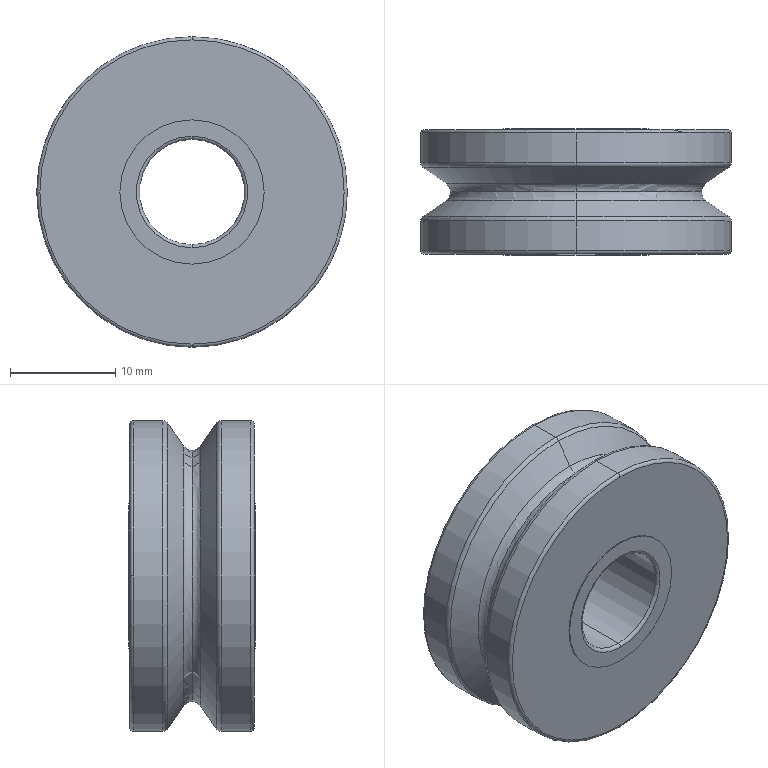Part | SolidWorks | features BaseBody 1 | 1 solid | 34 faces | box 29.5 x 12 x 29.5 mm | volume 6423 mm3 | torus 16 | cylinder 10 | cone 4 | plane 4 | commonest cylinder face diameters 13.7 x4 29.5 x4 10 x2
STEP:
#1=CARTESIAN_POINT('',(0.,-0.8192,-12.35));
#2=VERTEX_POINT('',#1);
#3=CARTESIAN_POINT('',(0.,0.,-11.923));
#4=VERTEX_POINT('',#3);
#5=CARTESIAN_POINT('',(0.,0.,-12.923));
#6=DIRECTION('',(-1.,0.,0.));
#7=DIRECTION('',(0.,0.,1.));
#8=AXIS2_PLACEMENT_3D('',#5,#6,#7);
#9=CIRCLE('',#8,1.);
#10=EDGE_CURVE('',#2,#4,#9,.T.);
#11=ORIENTED_EDGE('',*,*,#10,.T.);
#12=CARTESIAN_POINT('',(0.,0.,11.923));
#13=VERTEX_POINT('',#12);
#14=CARTESIAN_POINT('',(0.,0.,0.));
#15=DIRECTION('',(0.,-1.,0.));
#16=DIRECTION('',(0.,0.,-1.));
#17=AXIS2_PLACEMENT_3D('',#14,#15,#16);
#18=CIRCLE('',#17,11.923);
#19=EDGE_CURVE('',#4,#13,#18,.T.);
#20=ORIENTED_EDGE('',*,*,#19,.T.);
#21=CARTESIAN_POINT('',(0.,-0.8192,12.35));
#22=VERTEX_POINT('',#21);
#23=CARTESIAN_POINT('',(0.,0.,12.923));
#24=DIRECTION('',(1.,0.,0.));
#25=DIRECTION('',(0.,0.,-1.));
#26=AXIS2_PLACEMENT_3D('',#23,#24,#25);
#27=CIRCLE('',#26,1.);
#28=EDGE_CURVE('',#22,#13,#27,.T.);
#29=ORIENTED_EDGE('',*,*,#28,.F.);
#30=CARTESIAN_POINT('',(0.,-0.8192,0.));
#31=DIRECTION('',(0.,-1.,0.));
#32=DIRECTION('',(0.,0.,-1.));
#33=AXIS2_PLACEMENT_3D('',#30,#31,#32);
#34=CIRCLE('',#33,12.35);
#35=EDGE_CURVE('',#2,#22,#34,.T.);
#36=ORIENTED_EDGE('',*,*,#35,.F.);
#37=EDGE_LOOP('',(#11,#20,#29,#36));
#38=FACE_OUTER_BOUND('',#37,.T.);
#39=CARTESIAN_POINT('',(0.,0.,0.));
#40=DIRECTION('',(0.,-1.,0.));
#41=DIRECTION('',(0.,0.,-1.));
#42=AXIS2_PLACEMENT_3D('',#39,#40,#41);
#43=TOROIDAL_SURFACE('',#42,12.923,1.);
#44=ADVANCED_FACE('',(#38),#43,.F.);
#45=ORIENTED_EDGE('',*,*,#28,.T.);
#46=CARTESIAN_POINT('',(0.,0.,0.));
#47=DIRECTION('',(0.,-1.,0.));
#48=DIRECTION('',(0.,0.,-1.));
#49=AXIS2_PLACEMENT_3D('',#46,#47,#48);
#50=CIRCLE('',#49,11.923);
#51=EDGE_CURVE('',#13,#4,#50,.T.);
#52=ORIENTED_EDGE('',*,*,#51,.T.);
#53=ORIENTED_EDGE('',*,*,#10,.F.);
#54=CARTESIAN_POINT('',(0.,-0.8192,0.));
#55=DIRECTION('',(0.,-1.,0.));
#56=DIRECTION('',(0.,0.,-1.));
#57=AXIS2_PLACEMENT_3D('',#54,#55,#56);
#58=CIRCLE('',#57,12.35);
#59=EDGE_CURVE('',#22,#2,#58,.T.);
#60=ORIENTED_EDGE('',*,*,#59,.F.);
#61=EDGE_LOOP('',(#45,#52,#53,#60));
#62=FACE_OUTER_BOUND('',#61,.T.);
#63=CARTESIAN_POINT('',(0.,0.,0.));
#64=DIRECTION('',(0.,-1.,0.));
#65=DIRECTION('',(0.,0.,-1.));
#66=AXIS2_PLACEMENT_3D('',#63,#64,#65);
#67=TOROIDAL_SURFACE('',#66,12.923,1.);
#68=ADVANCED_FACE('',(#62),#67,.F.);
#69=CARTESIAN_POINT('',(0.,5.9,14.45));
#70=VERTEX_POINT('',#69);
#71=CARTESIAN_POINT('',(-14.45,5.9,0.));
#72=VERTEX_POINT('',#71);
#73=CARTESIAN_POINT('',(0.,5.9,0.));
#74=DIRECTION('',(0.,-1.,0.));
#75=DIRECTION('',(1.,0.,0.));
#76=AXIS2_PLACEMENT_3D('',#73,#74,#75);
#77=CIRCLE('',#76,14.45);
#78=EDGE_CURVE('',#70,#72,#77,.T.);
#79=ORIENTED_EDGE('',*,*,#78,.T.);
#80=CARTESIAN_POINT('',(-14.75,5.6,0.));
#81=VERTEX_POINT('',#80);
#82=CARTESIAN_POINT('',(-14.45,5.6,0.));
#83=DIRECTION('',(0.,0.,1.));
#84=DIRECTION('',(1.,0.,0.));
#85=AXIS2_PLACEMENT_3D('',#82,#83,#84);
#86=CIRCLE('',#85,0.3);
#87=EDGE_CURVE('',#72,#81,#86,.T.);
#88=ORIENTED_EDGE('',*,*,#87,.T.);
#89=CARTESIAN_POINT('',(0.,5.6,14.75));
#90=VERTEX_POINT('',#89);
#91=CARTESIAN_POINT('',(0.,5.6,0.));
#92=DIRECTION('',(0.,1.,0.));
#93=DIRECTION('',(-1.,0.,0.));
#94=AXIS2_PLACEMENT_3D('',#91,#92,#93);
#95=CIRCLE('',#94,14.75);
#96=EDGE_CURVE('',#81,#90,#95,.T.);
#97=ORIENTED_EDGE('',*,*,#96,.T.);
#98=CARTESIAN_POINT('',(14.75,5.6,0.));
#99=VERTEX_POINT('',#98);
#100=CARTESIAN_POINT('',(0.,5.6,0.));
#101=DIRECTION('',(0.,1.,0.));
#102=DIRECTION('',(-1.,0.,0.));
#103=AXIS2_PLACEMENT_3D('',#100,#101,#102);
#104=CIRCLE('',#103,14.75);
#105=EDGE_CURVE('',#90,#99,#104,.T.);
#106=ORIENTED_EDGE('',*,*,#105,.T.);
#107=CARTESIAN_POINT('',(14.45,5.9,-0.000000115));
#108=VERTEX_POINT('',#107);
#109=CARTESIAN_POINT('',(14.45,5.6,0.));
#110=DIRECTION('',(0.,0.,-1.));
#111=DIRECTION('',(0.,1.,0.));
#112=AXIS2_PLACEMENT_3D('',#109,#110,#111);
#113=CIRCLE('',#112,0.3);
#114=EDGE_CURVE('',#108,#99,#113,.T.);
#115=ORIENTED_EDGE('',*,*,#114,.F.);
#116=CARTESIAN_POINT('',(14.45,5.9,-0.000000115));
#117=CARTESIAN_POINT('',(14.45,5.9,0.00255));
#118=CARTESIAN_POINT('',(14.45,5.9,0.007389));
#119=CARTESIAN_POINT('',(14.45,5.9,0.01478));
#120=CARTESIAN_POINT('',(14.45,5.9,0.02586));
#121=CARTESIAN_POINT('',(14.45,5.9,0.05172));
#122=CARTESIAN_POINT('',(14.45,5.9,0.1034));
#123=CARTESIAN_POINT('',(14.449,5.9,0.2069));
#124=CARTESIAN_POINT('',(14.445,5.9,0.4137));
#125=CARTESIAN_POINT('',(14.43,5.9,0.8272));
#126=CARTESIAN_POINT('',(14.404,5.9,1.181));
#127=CARTESIAN_POINT('',(14.334,5.9,1.887));
#128=CARTESIAN_POINT('',(14.265,5.9,2.355));
#129=CARTESIAN_POINT('',(13.988,5.9,3.747));
#130=CARTESIAN_POINT('',(13.712,5.9,4.656));
#131=CARTESIAN_POINT('',(12.626,5.9,7.277));
#132=CARTESIAN_POINT('',(11.555,5.9,8.88));
#133=CARTESIAN_POINT('',(8.88,5.9,11.555));
#134=CARTESIAN_POINT('',(7.277,5.9,12.626));
#135=CARTESIAN_POINT('',(3.782,5.9,14.074));
#136=CARTESIAN_POINT('',(1.892,5.9,14.45));
#137=CARTESIAN_POINT('',(0.,5.9,14.45));
#138=B_SPLINE_CURVE_WITH_KNOTS('',3,(#116,#117,#118,#119,#120,#121,#122,#123,#124,#125,#126,#127,#128,#129,#130,#131,#132,#133,#134,#135,#136,#137),.UNSPECIFIED.,.F.,.F.,(4,2,1,1,1,1,1,1,2,2,2,2,2,4),(0.5,0.5002,0.5005,0.501,0.502,0.5039,0.5078,0.5156,0.5312,0.5625,0.625,0.75,0.875,1.),.UNSPECIFIED.);
#139=EDGE_CURVE('',#108,#70,#138,.T.);
#140=ORIENTED_EDGE('',*,*,#139,.T.);
#141=EDGE_LOOP('',(#79,#88,#97,#106,#115,#140));
#142=FACE_OUTER_BOUND('',#141,.T.);
#143=CARTESIAN_POINT('',(0.,5.6,0.));
#144=DIRECTION('',(0.,-1.,0.));
#145=DIRECTION('',(1.,0.,0.));
#146=AXIS2_PLACEMENT_3D('',#143,#144,#145);
#147=TOROIDAL_SURFACE('',#146,14.45,0.3);
#148=ADVANCED_FACE('',(#142),#147,.T.);
#149=CARTESIAN_POINT('',(0.,6.,-6.85));
#150=VERTEX_POINT('',#149);
#151=CARTESIAN_POINT('',(0.,6.,6.85));
#152=VERTEX_POINT('',#151);
#153=CARTESIAN_POINT('',(0.,6.,0.));
#154=DIRECTION('',(0.,-1.,0.));
#155=DIRECTION('',(0.,0.,-1.));
#156=AXIS2_PLACEMENT_3D('',#153,#154,#155);
#157=CIRCLE('',#156,6.85);
#158=EDGE_CURVE('',#150,#152,#157,.T.);
#159=ORIENTED_EDGE('',*,*,#158,.T.);
#160=CARTESIAN_POINT('',(0.,5.9,6.85));
#161=VERTEX_POINT('',#160);
#162=CARTESIAN_POINT('',(0.,0.,6.85));
#163=DIRECTION('',(0.,-1.,0.));
#164=VECTOR('',#163,1000.);
#165=LINE('',#162,#164);
#166=EDGE_CURVE('',#152,#161,#165,.T.);
#167=ORIENTED_EDGE('',*,*,#166,.T.);
#168=CARTESIAN_POINT('',(0.,5.9,-6.85));
#169=VERTEX_POINT('',#168);
#170=CARTESIAN_POINT('',(0.,5.9,0.));
#171=DIRECTION('',(0.,1.,0.));
#172=DIRECTION('',(0.,0.,-1.));
#173=AXIS2_PLACEMENT_3D('',#170,#171,#172);
#174=CIRCLE('',#173,6.85);
#175=EDGE_CURVE('',#161,#169,#174,.T.);
#176=ORIENTED_EDGE('',*,*,#175,.T.);
#177=CARTESIAN_POINT('',(0.,0.,-6.85));
#178=DIRECTION('',(0.,-1.,0.));
#179=VECTOR('',#178,1000.);
#180=LINE('',#177,#179);
#181=EDGE_CURVE('',#150,#169,#180,.T.);
#182=ORIENTED_EDGE('',*,*,#181,.F.);
#183=EDGE_LOOP('',(#159,#167,#176,#182));
#184=FACE_OUTER_BOUND('',#183,.T.);
#185=CARTESIAN_POINT('',(0.,0.,0.));
#186=DIRECTION('',(0.,-1.,0.));
#187=DIRECTION('',(0.,0.,-1.));
#188=AXIS2_PLACEMENT_3D('',#185,#186,#187);
#189=CYLINDRICAL_SURFACE('',#188,6.85);
#190=ADVANCED_FACE('',(#184),#189,.T.);
#191=ORIENTED_EDGE('',*,*,#105,.F.);
#192=CARTESIAN_POINT('',(0.,2.76,14.75));
#193=VERTEX_POINT('',#192);
#194=CARTESIAN_POINT('',(0.,0.,14.75));
#195=DIRECTION('',(0.,-1.,0.));
#196=VECTOR('',#195,1000.);
#197=LINE('',#194,#196);
#198=EDGE_CURVE('',#90,#193,#197,.T.);
#199=ORIENTED_EDGE('',*,*,#198,.T.);
#200=CARTESIAN_POINT('',(0.,2.76,-14.75));
#201=VERTEX_POINT('',#200);
#202=CARTESIAN_POINT('',(0.,2.76,0.));
#203=DIRECTION('',(0.,1.,0.));
#204=DIRECTION('',(0.,0.,-1.));
#205=AXIS2_PLACEMENT_3D('',#202,#203,#204);
#206=CIRCLE('',#205,14.75);
#207=EDGE_CURVE('',#193,#201,#206,.T.);
#208=ORIENTED_EDGE('',*,*,#207,.T.);
#209=CARTESIAN_POINT('',(0.,5.6,-14.75));
#210=VERTEX_POINT('',#209);
#211=CARTESIAN_POINT('',(0.,0.,-14.75));
#212=DIRECTION('',(0.,-1.,0.));
#213=VECTOR('',#212,1000.);
#214=LINE('',#211,#213);
#215=EDGE_CURVE('',#210,#201,#214,.T.);
#216=ORIENTED_EDGE('',*,*,#215,.F.);
#217=CARTESIAN_POINT('',(0.,5.6,0.));
#218=DIRECTION('',(0.,1.,0.));
#219=DIRECTION('',(-1.,0.,0.));
#220=AXIS2_PLACEMENT_3D('',#217,#218,#219);
#221=CIRCLE('',#220,14.75);
#222=EDGE_CURVE('',#99,#210,#221,.T.);
#223=ORIENTED_EDGE('',*,*,#222,.F.);
#224=EDGE_LOOP('',(#191,#199,#208,#216,#223));
#225=FACE_OUTER_BOUND('',#224,.T.);
#226=CARTESIAN_POINT('',(0.,0.,0.));
#227=DIRECTION('',(0.,-1.,0.));
#228=DIRECTION('',(0.,0.,-1.));
#229=AXIS2_PLACEMENT_3D('',#226,#227,#228);
#230=CYLINDRICAL_SURFACE('',#229,14.75);
#231=ADVANCED_FACE('',(#225),#230,.T.);
#232=ORIENTED_EDGE('',*,*,#207,.F.);
#233=CARTESIAN_POINT('',(0.,2.351,14.537));
#234=VERTEX_POINT('',#233);
#235=CARTESIAN_POINT('',(0.,2.76,14.25));
#236=DIRECTION('',(1.,0.,0.));
#237=DIRECTION('',(0.,0.,-1.));
#238=AXIS2_PLACEMENT_3D('',#235,#236,#237);
#239=CIRCLE('',#238,0.5);
#240=EDGE_CURVE('',#193,#234,#239,.T.);
#241=ORIENTED_EDGE('',*,*,#240,.T.);
#242=CARTESIAN_POINT('',(0.,2.351,-14.537));
#243=VERTEX_POINT('',#242);
#244=CARTESIAN_POINT('',(0.,2.351,0.));
#245=DIRECTION('',(0.,1.,0.));
#246=DIRECTION('',(0.,0.,1.));
#247=AXIS2_PLACEMENT_3D('',#244,#245,#246);
#248=CIRCLE('',#247,14.537);
#249=EDGE_CURVE('',#234,#243,#248,.T.);
#250=ORIENTED_EDGE('',*,*,#249,.T.);
#251=CARTESIAN_POINT('',(0.,2.76,-14.25));
#252=DIRECTION('',(-1.,0.,0.));
#253=DIRECTION('',(0.,0.,1.));
#254=AXIS2_PLACEMENT_3D('',#251,#252,#253);
#255=CIRCLE('',#254,0.5);
#256=EDGE_CURVE('',#201,#243,#255,.T.);
#257=ORIENTED_EDGE('',*,*,#256,.F.);
#258=EDGE_LOOP('',(#232,#241,#250,#257));
#259=FACE_OUTER_BOUND('',#258,.T.);
#260=CARTESIAN_POINT('',(0.,2.76,0.));
#261=DIRECTION('',(0.,-1.,0.));
#262=DIRECTION('',(0.,0.,-1.));
#263=AXIS2_PLACEMENT_3D('',#260,#261,#262);
#264=TOROIDAL_SURFACE('',#263,14.25,0.5);
#265=ADVANCED_FACE('',(#259),#264,.T.);
#266=CARTESIAN_POINT('',(0.,5.7,-5.));
#267=VERTEX_POINT('',#266);
#268=CARTESIAN_POINT('',(0.,5.7,5.));
#269=VERTEX_POINT('',#268);
#270=CARTESIAN_POINT('',(0.,5.7,0.));
#271=DIRECTION('',(0.,-1.,0.));
#272=DIRECTION('',(1.,0.,0.));
#273=AXIS2_PLACEMENT_3D('',#270,#271,#272);
#274=CIRCLE('',#273,5.);
#275=EDGE_CURVE('',#267,#269,#274,.T.);
#276=ORIENTED_EDGE('',*,*,#275,.T.);
#277=CARTESIAN_POINT('',(0.,6.,5.3));
#278=VERTEX_POINT('',#277);
#279=CARTESIAN_POINT('',(0.,5.7,5.3));
#280=DIRECTION('',(1.,0.,0.));
#281=DIRECTION('',(0.,0.,-1.));
#282=AXIS2_PLACEMENT_3D('',#279,#280,#281);
#283=CIRCLE('',#282,0.3);
#284=EDGE_CURVE('',#269,#278,#283,.T.);
#285=ORIENTED_EDGE('',*,*,#284,.T.);
#286=CARTESIAN_POINT('',(0.,6.,-5.3));
#287=VERTEX_POINT('',#286);
#288=CARTESIAN_POINT('',(0.,6.,0.));
#289=DIRECTION('',(0.,1.,0.));
#290=DIRECTION('',(0.,0.,-1.));
#291=AXIS2_PLACEMENT_3D('',#288,#289,#290);
#292=CIRCLE('',#291,5.3);
#293=EDGE_CURVE('',#278,#287,#292,.T.);
#294=ORIENTED_EDGE('',*,*,#293,.T.);
#295=CARTESIAN_POINT('',(0.,5.7,-5.3));
#296=DIRECTION('',(-1.,0.,0.));
#297=DIRECTION('',(0.,0.,1.));
#298=AXIS2_PLACEMENT_3D('',#295,#296,#297);
#299=CIRCLE('',#298,0.3);
#300=EDGE_CURVE('',#267,#287,#299,.T.);
#301=ORIENTED_EDGE('',*,*,#300,.F.);
#302=EDGE_LOOP('',(#276,#285,#294,#301));
#303=FACE_OUTER_BOUND('',#302,.T.);
#304=CARTESIAN_POINT('',(0.,5.7,0.));
#305=DIRECTION('',(0.,-1.,0.));
#306=DIRECTION('',(0.,0.,-1.));
#307=AXIS2_PLACEMENT_3D('',#304,#305,#306);
#308=TOROIDAL_SURFACE('',#307,5.3,0.3);
#309=ADVANCED_FACE('',(#303),#308,.T.);
#310=CARTESIAN_POINT('',(0.,0.8192,12.35));
#311=VERTEX_POINT('',#310);
#312=CARTESIAN_POINT('',(0.,0.8192,-12.35));
#313=VERTEX_POINT('',#312);
#314=CARTESIAN_POINT('',(0.,0.8192,0.));
#315=DIRECTION('',(0.,1.,0.));
#316=DIRECTION('',(0.,0.,1.));
#317=AXIS2_PLACEMENT_3D('',#314,#315,#316);
#318=CIRCLE('',#317,12.35);
#319=EDGE_CURVE('',#311,#313,#318,.T.);
#320=ORIENTED_EDGE('',*,*,#319,.T.);
#321=CARTESIAN_POINT('',(0.,2.351,-14.537));
#322=DIRECTION('',(0.,0.5736,-0.8192));
#323=VECTOR('',#322,1000.);
#324=LINE('',#321,#323);
#325=EDGE_CURVE('',#313,#243,#324,.T.);
#326=ORIENTED_EDGE('',*,*,#325,.T.);
#327=ORIENTED_EDGE('',*,*,#249,.F.);
#328=CARTESIAN_POINT('',(0.,2.351,14.537));
#329=DIRECTION('',(0.,0.5736,0.8192));
#330=VECTOR('',#329,1000.);
#331=LINE('',#328,#330);
#332=EDGE_CURVE('',#311,#234,#331,.T.);
#333=ORIENTED_EDGE('',*,*,#332,.F.);
#334=EDGE_LOOP('',(#320,#326,#327,#333));
#335=FACE_OUTER_BOUND('',#334,.T.);
#336=CARTESIAN_POINT('',(0.,2.351,0.));
#337=DIRECTION('',(0.,1.,0.));
#338=DIRECTION('',(0.,0.,1.));
#339=AXIS2_PLACEMENT_3D('',#336,#337,#338);
#340=CONICAL_SURFACE('',#339,14.537,0.9599);
#341=ADVANCED_FACE('',(#335),#340,.T.);
#342=CARTESIAN_POINT('',(0.,5.7,0.));
#343=DIRECTION('',(0.,-1.,0.));
#344=DIRECTION('',(1.,0.,0.));
#345=AXIS2_PLACEMENT_3D('',#342,#343,#344);
#346=CIRCLE('',#345,5.);
#347=EDGE_CURVE('',#269,#267,#346,.T.);
#348=ORIENTED_EDGE('',*,*,#347,.F.);
#349=CARTESIAN_POINT('',(0.,-5.7,5.));
#350=VERTEX_POINT('',#349);
#351=CARTESIAN_POINT('',(0.,0.,5.));
#352=DIRECTION('',(0.,-1.,0.));
#353=VECTOR('',#352,1000.);
#354=LINE('',#351,#353);
#355=EDGE_CURVE('',#269,#350,#354,.T.);
#356=ORIENTED_EDGE('',*,*,#355,.T.);
#357=CARTESIAN_POINT('',(0.,-5.7,-5.));
#358=VERTEX_POINT('',#357);
#359=CARTESIAN_POINT('',(0.,-5.7,0.));
#360=DIRECTION('',(0.,1.,0.));
#361=DIRECTION('',(0.,0.,-1.));
#362=AXIS2_PLACEMENT_3D('',#359,#360,#361);
#363=CIRCLE('',#362,5.);
#364=EDGE_CURVE('',#358,#350,#363,.T.);
#365=ORIENTED_EDGE('',*,*,#364,.F.);
#366=CARTESIAN_POINT('',(0.,0.,-5.));
#367=DIRECTION('',(0.,-1.,0.));
#368=VECTOR('',#367,1000.);
#369=LINE('',#366,#368);
#370=EDGE_CURVE('',#267,#358,#369,.T.);
#371=ORIENTED_EDGE('',*,*,#370,.F.);
#372=EDGE_LOOP('',(#348,#356,#365,#371));
#373=FACE_OUTER_BOUND('',#372,.T.);
#374=CARTESIAN_POINT('',(0.,0.,0.));
#375=DIRECTION('',(0.,-1.,0.));
#376=DIRECTION('',(0.,0.,-1.));
#377=AXIS2_PLACEMENT_3D('',#374,#375,#376);
#378=CYLINDRICAL_SURFACE('',#377,5.);
#379=ADVANCED_FACE('',(#373),#378,.F.);
#380=ORIENTED_EDGE('',*,*,#51,.F.);
#381=CARTESIAN_POINT('',(0.,0.,12.923));
#382=DIRECTION('',(1.,0.,0.));
#383=DIRECTION('',(0.,0.,-1.));
#384=AXIS2_PLACEMENT_3D('',#381,#382,#383);
#385=CIRCLE('',#384,1.);
#386=EDGE_CURVE('',#13,#311,#385,.T.);
#387=ORIENTED_EDGE('',*,*,#386,.T.);
#388=CARTESIAN_POINT('',(0.,0.8192,0.));
#389=DIRECTION('',(0.,1.,0.));
#390=DIRECTION('',(0.,0.,1.));
#391=AXIS2_PLACEMENT_3D('',#388,#389,#390);
#392=CIRCLE('',#391,12.35);
#393=EDGE_CURVE('',#313,#311,#392,.T.);
#394=ORIENTED_EDGE('',*,*,#393,.F.);
#395=CARTESIAN_POINT('',(0.,0.,-12.923));
#396=DIRECTION('',(-1.,0.,0.));
#397=DIRECTION('',(0.,0.,1.));
#398=AXIS2_PLACEMENT_3D('',#395,#396,#397);
#399=CIRCLE('',#398,1.);
#400=EDGE_CURVE('',#4,#313,#399,.T.);
#401=ORIENTED_EDGE('',*,*,#400,.F.);
#402=EDGE_LOOP('',(#380,#387,#394,#401));
#403=FACE_OUTER_BOUND('',#402,.T.);
#404=CARTESIAN_POINT('',(0.,0.,0.));
#405=DIRECTION('',(0.,-1.,0.));
#406=DIRECTION('',(0.,0.,-1.));
#407=AXIS2_PLACEMENT_3D('',#404,#405,#406);
#408=TOROIDAL_SURFACE('',#407,12.923,1.);
#409=ADVANCED_FACE('',(#403),#408,.F.);
#410=CARTESIAN_POINT('',(0.,-5.7,0.));
#411=DIRECTION('',(0.,1.,0.));
#412=DIRECTION('',(0.,0.,-1.));
#413=AXIS2_PLACEMENT_3D('',#410,#411,#412);
#414=CIRCLE('',#413,5.);
#415=EDGE_CURVE('',#350,#358,#414,.T.);
#416=ORIENTED_EDGE('',*,*,#415,.T.);
#417=CARTESIAN_POINT('',(0.,-6.,-5.3));
#418=VERTEX_POINT('',#417);
#419=CARTESIAN_POINT('',(0.,-5.7,-5.3));
#420=DIRECTION('',(1.,0.,0.));
#421=DIRECTION('',(0.,0.,-1.));
#422=AXIS2_PLACEMENT_3D('',#419,#420,#421);
#423=CIRCLE('',#422,0.3);
#424=EDGE_CURVE('',#358,#418,#423,.T.);
#425=ORIENTED_EDGE('',*,*,#424,.T.);
#426=CARTESIAN_POINT('',(0.,-6.,5.3));
#427=VERTEX_POINT('',#426);
#428=CARTESIAN_POINT('',(0.,-6.,0.));
#429=DIRECTION('',(0.,-1.,0.));
#430=DIRECTION('',(0.,0.,1.));
#431=AXIS2_PLACEMENT_3D('',#428,#429,#430);
#432=CIRCLE('',#431,5.3);
#433=EDGE_CURVE('',#418,#427,#432,.T.);
#434=ORIENTED_EDGE('',*,*,#433,.T.);
#435=CARTESIAN_POINT('',(0.,-5.7,5.3));
#436=DIRECTION('',(-1.,0.,0.));
#437=DIRECTION('',(0.,0.,1.));
#438=AXIS2_PLACEMENT_3D('',#435,#436,#437);
#439=CIRCLE('',#438,0.3);
#440=EDGE_CURVE('',#350,#427,#439,.T.);
#441=ORIENTED_EDGE('',*,*,#440,.F.);
#442=EDGE_LOOP('',(#416,#425,#434,#441));
#443=FACE_OUTER_BOUND('',#442,.T.);
#444=CARTESIAN_POINT('',(0.,-5.7,0.));
#445=DIRECTION('',(0.,1.,0.));
#446=DIRECTION('',(0.,0.,1.));
#447=AXIS2_PLACEMENT_3D('',#444,#445,#446);
#448=TOROIDAL_SURFACE('',#447,5.3,0.3);
#449=ADVANCED_FACE('',(#443),#448,.T.);
#450=ORIENTED_EDGE('',*,*,#35,.T.);
#451=CARTESIAN_POINT('',(0.,-2.351,14.537));
#452=VERTEX_POINT('',#451);
#453=CARTESIAN_POINT('',(0.,-2.351,14.537));
#454=DIRECTION('',(0.,-0.5736,0.8192));
#455=VECTOR('',#454,1000.);
#456=LINE('',#453,#455);
#457=EDGE_CURVE('',#22,#452,#456,.T.);
#458=ORIENTED_EDGE('',*,*,#457,.T.);
#459=CARTESIAN_POINT('',(0.,-2.351,-14.537));
#460=VERTEX_POINT('',#459);
#461=CARTESIAN_POINT('',(0.,-2.351,0.));
#462=DIRECTION('',(0.,1.,0.));
#463=DIRECTION('',(1.,0.,0.));
#464=AXIS2_PLACEMENT_3D('',#461,#462,#463);
#465=CIRCLE('',#464,14.537);
#466=EDGE_CURVE('',#452,#460,#465,.T.);
#467=ORIENTED_EDGE('',*,*,#466,.T.);
#468=CARTESIAN_POINT('',(0.,-2.351,-14.537));
#469=DIRECTION('',(0.,-0.5736,-0.8192));
#470=VECTOR('',#469,1000.);
#471=LINE('',#468,#470);
#472=EDGE_CURVE('',#2,#460,#471,.T.);
#473=ORIENTED_EDGE('',*,*,#472,.F.);
#474=EDGE_LOOP('',(#450,#458,#467,#473));
#475=FACE_OUTER_BOUND('',#474,.T.);
#476=CARTESIAN_POINT('',(0.,-2.351,0.));
#477=DIRECTION('',(0.,-1.,0.));
#478=DIRECTION('',(0.,0.,-1.));
#479=AXIS2_PLACEMENT_3D('',#476,#477,#478);
#480=CONICAL_SURFACE('',#479,14.537,0.9599);
#481=ADVANCED_FACE('',(#475),#480,.T.);
#482=ORIENTED_EDGE('',*,*,#466,.F.);
#483=CARTESIAN_POINT('',(0.,-2.76,14.75));
#484=VERTEX_POINT('',#483);
#485=CARTESIAN_POINT('',(0.,-2.76,14.25));
#486=DIRECTION('',(1.,0.,0.));
#487=DIRECTION('',(0.,0.,-1.));
#488=AXIS2_PLACEMENT_3D('',#485,#486,#487);
#489=CIRCLE('',#488,0.5);
#490=EDGE_CURVE('',#452,#484,#489,.T.);
#491=ORIENTED_EDGE('',*,*,#490,.T.);
#492=CARTESIAN_POINT('',(0.,-2.76,-14.75));
#493=VERTEX_POINT('',#492);
#494=CARTESIAN_POINT('',(0.,-2.76,0.));
#495=DIRECTION('',(0.,1.,0.));
#496=DIRECTION('',(0.,0.,1.));
#497=AXIS2_PLACEMENT_3D('',#494,#495,#496);
#498=CIRCLE('',#497,14.75);
#499=EDGE_CURVE('',#484,#493,#498,.T.);
#500=ORIENTED_EDGE('',*,*,#499,.T.);
#501=CARTESIAN_POINT('',(0.,-2.76,-14.25));
#502=DIRECTION('',(-1.,0.,0.));
#503=DIRECTION('',(0.,0.,1.));
#504=AXIS2_PLACEMENT_3D('',#501,#502,#503);
#505=CIRCLE('',#504,0.5);
#506=EDGE_CURVE('',#460,#493,#505,.T.);
#507=ORIENTED_EDGE('',*,*,#506,.F.);
#508=EDGE_LOOP('',(#482,#491,#500,#507));
#509=FACE_OUTER_BOUND('',#508,.T.);
#510=CARTESIAN_POINT('',(0.,-2.76,0.));
#511=DIRECTION('',(0.,-1.,0.));
#512=DIRECTION('',(0.,0.,-1.));
#513=AXIS2_PLACEMENT_3D('',#510,#511,#512);
#514=TOROIDAL_SURFACE('',#513,14.25,0.5);
#515=ADVANCED_FACE('',(#509),#514,.T.);
#516=CARTESIAN_POINT('',(0.,-5.9,-6.85));
#517=VERTEX_POINT('',#516);
#518=CARTESIAN_POINT('',(0.,-5.9,6.85));
#519=VERTEX_POINT('',#518);
#520=CARTESIAN_POINT('',(0.,-5.9,0.));
#521=DIRECTION('',(0.,-1.,0.));
#522=DIRECTION('',(0.,0.,-1.));
#523=AXIS2_PLACEMENT_3D('',#520,#521,#522);
#524=CIRCLE('',#523,6.85);
#525=EDGE_CURVE('',#517,#519,#524,.T.);
#526=ORIENTED_EDGE('',*,*,#525,.T.);
#527=CARTESIAN_POINT('',(0.,-6.,6.85));
#528=VERTEX_POINT('',#527);
#529=CARTESIAN_POINT('',(0.,0.,6.85));
#530=DIRECTION('',(0.,-1.,0.));
#531=VECTOR('',#530,1000.);
#532=LINE('',#529,#531);
#533=EDGE_CURVE('',#519,#528,#532,.T.);
#534=ORIENTED_EDGE('',*,*,#533,.T.);
#535=CARTESIAN_POINT('',(0.,-6.,-6.85));
#536=VERTEX_POINT('',#535);
#537=CARTESIAN_POINT('',(0.,-6.,0.));
#538=DIRECTION('',(0.,1.,0.));
#539=DIRECTION('',(0.,0.,-1.));
#540=AXIS2_PLACEMENT_3D('',#537,#538,#539);
#541=CIRCLE('',#540,6.85);
#542=EDGE_CURVE('',#528,#536,#541,.T.);
#543=ORIENTED_EDGE('',*,*,#542,.T.);
#544=CARTESIAN_POINT('',(0.,0.,-6.85));
#545=DIRECTION('',(0.,-1.,0.));
#546=VECTOR('',#545,1000.);
#547=LINE('',#544,#546);
#548=EDGE_CURVE('',#517,#536,#547,.T.);
#549=ORIENTED_EDGE('',*,*,#548,.F.);
#550=EDGE_LOOP('',(#526,#534,#543,#549));
#551=FACE_OUTER_BOUND('',#550,.T.);
#552=CARTESIAN_POINT('',(0.,0.,0.));
#553=DIRECTION('',(0.,-1.,0.));
#554=DIRECTION('',(0.,0.,-1.));
#555=AXIS2_PLACEMENT_3D('',#552,#553,#554);
#556=CYLINDRICAL_SURFACE('',#555,6.85);
#557=ADVANCED_FACE('',(#551),#556,.T.);
#558=ORIENTED_EDGE('',*,*,#499,.F.);
#559=CARTESIAN_POINT('',(0.,-5.6,14.75));
#560=VERTEX_POINT('',#559);
#561=CARTESIAN_POINT('',(0.,0.,14.75));
#562=DIRECTION('',(0.,-1.,0.));
#563=VECTOR('',#562,1000.);
#564=LINE('',#561,#563);
#565=EDGE_CURVE('',#484,#560,#564,.T.);
#566=ORIENTED_EDGE('',*,*,#565,.T.);
#567=CARTESIAN_POINT('',(0.,-5.6,-14.75));
#568=VERTEX_POINT('',#567);
#569=CARTESIAN_POINT('',(0.,-5.6,0.));
#570=DIRECTION('',(0.,1.,0.));
#571=DIRECTION('',(0.,0.,-1.));
#572=AXIS2_PLACEMENT_3D('',#569,#570,#571);
#573=CIRCLE('',#572,14.75);
#574=EDGE_CURVE('',#560,#568,#573,.T.);
#575=ORIENTED_EDGE('',*,*,#574,.T.);
#576=CARTESIAN_POINT('',(0.,0.,-14.75));
#577=DIRECTION('',(0.,-1.,0.));
#578=VECTOR('',#577,1000.);
#579=LINE('',#576,#578);
#580=EDGE_CURVE('',#493,#568,#579,.T.);
#581=ORIENTED_EDGE('',*,*,#580,.F.);
#582=EDGE_LOOP('',(#558,#566,#575,#581));
#583=FACE_OUTER_BOUND('',#582,.T.);
#584=CARTESIAN_POINT('',(0.,0.,0.));
#585=DIRECTION('',(0.,-1.,0.));
#586=DIRECTION('',(0.,0.,-1.));
#587=AXIS2_PLACEMENT_3D('',#584,#585,#586);
#588=CYLINDRICAL_SURFACE('',#587,14.75);
#589=ADVANCED_FACE('',(#583),#588,.T.);
#590=CARTESIAN_POINT('',(0.,-5.9,14.45));
#591=VERTEX_POINT('',#590);
#592=CARTESIAN_POINT('',(0.,-5.9,-14.45));
#593=VERTEX_POINT('',#592);
#594=CARTESIAN_POINT('',(0.,-5.9,0.));
#595=DIRECTION('',(0.,1.,0.));
#596=DIRECTION('',(0.,0.,1.));
#597=AXIS2_PLACEMENT_3D('',#594,#595,#596);
#598=CIRCLE('',#597,14.45);
#599=EDGE_CURVE('',#591,#593,#598,.T.);
#600=ORIENTED_EDGE('',*,*,#599,.T.);
#601=CARTESIAN_POINT('',(0.,-5.6,-14.45));
#602=DIRECTION('',(1.,0.,0.));
#603=DIRECTION('',(0.,0.,-1.));
#604=AXIS2_PLACEMENT_3D('',#601,#602,#603);
#605=CIRCLE('',#604,0.3);
#606=EDGE_CURVE('',#593,#568,#605,.T.);
#607=ORIENTED_EDGE('',*,*,#606,.T.);
#608=ORIENTED_EDGE('',*,*,#574,.F.);
#609=CARTESIAN_POINT('',(0.,-5.6,14.45));
#610=DIRECTION('',(-1.,0.,0.));
#611=DIRECTION('',(0.,0.,1.));
#612=AXIS2_PLACEMENT_3D('',#609,#610,#611);
#613=CIRCLE('',#612,0.3);
#614=EDGE_CURVE('',#591,#560,#613,.T.);
#615=ORIENTED_EDGE('',*,*,#614,.F.);
#616=EDGE_LOOP('',(#600,#607,#608,#615));
#617=FACE_OUTER_BOUND('',#616,.T.);
#618=CARTESIAN_POINT('',(0.,-5.6,0.));
#619=DIRECTION('',(0.,1.,0.));
#620=DIRECTION('',(0.,0.,1.));
#621=AXIS2_PLACEMENT_3D('',#618,#619,#620);
#622=TOROIDAL_SURFACE('',#621,14.45,0.3);
#623=ADVANCED_FACE('',(#617),#622,.T.);
#624=ORIENTED_EDGE('',*,*,#78,.F.);
#625=ORIENTED_EDGE('',*,*,#139,.F.);
#626=CARTESIAN_POINT('',(0.,5.9,-14.45));
#627=VERTEX_POINT('',#626);
#628=CARTESIAN_POINT('',(0.,5.9,-14.45));
#629=CARTESIAN_POINT('',(0.6836,5.9,-14.45));
#630=CARTESIAN_POINT('',(1.367,5.9,-14.402));
#631=CARTESIAN_POINT('',(2.046,5.9,-14.305));
#632=CARTESIAN_POINT('',(2.045,5.9,-14.305));
#633=CARTESIAN_POINT('',(2.047,5.9,-14.305));
#634=CARTESIAN_POINT('',(2.05,5.9,-14.305));
#635=CARTESIAN_POINT('',(2.057,5.9,-14.304));
#636=CARTESIAN_POINT('',(2.072,5.9,-14.301));
#637=CARTESIAN_POINT('',(2.107,5.9,-14.296));
#638=CARTESIAN_POINT('',(2.144,5.9,-14.291));
#639=CARTESIAN_POINT('',(2.229,5.9,-14.278));
#640=CARTESIAN_POINT('',(2.3,5.9,-14.267));
#641=CARTESIAN_POINT('',(2.552,5.9,-14.225));
#642=CARTESIAN_POINT('',(2.774,5.9,-14.185));
#643=CARTESIAN_POINT('',(3.067,5.9,-14.121));
#644=CARTESIAN_POINT('',(3.08,5.9,-14.118));
#645=CARTESIAN_POINT('',(3.11,5.9,-14.112));
#646=CARTESIAN_POINT('',(3.155,5.9,-14.102));
#647=CARTESIAN_POINT('',(3.256,5.9,-14.079));
#648=CARTESIAN_POINT('',(3.337,5.9,-14.06));
#649=CARTESIAN_POINT('',(3.491,5.9,-14.023));
#650=CARTESIAN_POINT('',(3.583,5.9,-13.999));
#651=CARTESIAN_POINT('',(3.832,5.9,-13.934));
#652=CARTESIAN_POINT('',(3.958,5.9,-13.898));
#653=CARTESIAN_POINT('',(4.047,5.9,-13.872));
#654=CARTESIAN_POINT('',(4.052,5.9,-13.87));
#655=CARTESIAN_POINT('',(4.059,5.9,-13.868));
#656=CARTESIAN_POINT('',(4.069,5.9,-13.865));
#657=CARTESIAN_POINT('',(4.091,5.9,-13.859));
#658=CARTESIAN_POINT('',(4.137,5.9,-13.845));
#659=CARTESIAN_POINT('',(4.228,5.9,-13.818));
#660=CARTESIAN_POINT('',(4.409,5.9,-13.762));
#661=CARTESIAN_POINT('',(4.769,5.9,-13.643));
#662=CARTESIAN_POINT('',(5.074,5.9,-13.532));
#663=CARTESIAN_POINT('',(5.679,5.9,-13.295));
#664=CARTESIAN_POINT('',(6.075,5.9,-13.118));
#665=CARTESIAN_POINT('',(7.237,5.9,-12.537));
#666=CARTESIAN_POINT('',(7.977,5.9,-12.08));
#667=CARTESIAN_POINT('',(8.681,5.9,-11.552));
#668=CARTESIAN_POINT('',(8.695,5.9,-11.541));
#669=CARTESIAN_POINT('',(8.72,5.9,-11.522));
#670=CARTESIAN_POINT('',(8.758,5.9,-11.493));
#671=CARTESIAN_POINT('',(8.846,5.9,-11.426));
#672=CARTESIAN_POINT('',(9.02,5.9,-11.29));
#673=CARTESIAN_POINT('',(9.363,5.9,-11.012));
#674=CARTESIAN_POINT('',(9.836,5.9,-10.594));
#675=CARTESIAN_POINT('',(10.197,5.9,-10.241));
#676=CARTESIAN_POINT('',(10.417,5.9,-10.015));
#677=CARTESIAN_POINT('',(10.46,5.9,-9.97));
#678=CARTESIAN_POINT('',(10.552,5.9,-9.872));
#679=CARTESIAN_POINT('',(10.691,5.9,-9.723));
#680=CARTESIAN_POINT('',(10.826,5.9,-9.572));
#681=CARTESIAN_POINT('',(11.624,5.9,-8.652));
#682=CARTESIAN_POINT('',(12.241,5.9,-7.755));
#683=CARTESIAN_POINT('',(12.758,5.9,-6.785));
#684=CARTESIAN_POINT('',(12.767,5.9,-6.768));
#685=CARTESIAN_POINT('',(12.784,5.9,-6.736));
#686=CARTESIAN_POINT('',(12.809,5.9,-6.688));
#687=CARTESIAN_POINT('',(12.868,5.9,-6.575));
#688=CARTESIAN_POINT('',(12.982,5.9,-6.348));
#689=CARTESIAN_POINT('',(13.201,5.9,-5.889));
#690=CARTESIAN_POINT('',(13.371,5.9,-5.488));
#691=CARTESIAN_POINT('',(13.477,5.9,-5.215));
#692=CARTESIAN_POINT('',(13.476,5.9,-5.216));
#693=CARTESIAN_POINT('',(13.477,5.9,-5.214));
#694=CARTESIAN_POINT('',(13.478,5.9,-5.212));
#695=CARTESIAN_POINT('',(13.479,5.9,-5.208));
#696=CARTESIAN_POINT('',(13.483,5.9,-5.198));
#697=CARTESIAN_POINT('',(13.493,5.9,-5.173));
#698=CARTESIAN_POINT('',(13.503,5.9,-5.145));
#699=CARTESIAN_POINT('',(13.528,5.9,-5.081));
#700=CARTESIAN_POINT('',(13.549,5.9,-5.025));
#701=CARTESIAN_POINT('',(13.623,5.9,-4.821));
#702=CARTESIAN_POINT('',(13.689,5.9,-4.634));
#703=CARTESIAN_POINT('',(13.768,5.9,-4.389));
#704=CARTESIAN_POINT('',(13.769,5.9,-4.384));
#705=CARTESIAN_POINT('',(13.773,5.9,-4.371));
#706=CARTESIAN_POINT('',(13.779,5.9,-4.353));
#707=CARTESIAN_POINT('',(13.793,5.9,-4.31));
#708=CARTESIAN_POINT('',(13.818,5.9,-4.227));
#709=CARTESIAN_POINT('',(13.839,5.9,-4.16));
#710=CARTESIAN_POINT('',(13.877,5.9,-4.031));
#711=CARTESIAN_POINT('',(13.899,5.9,-3.953));
#712=CARTESIAN_POINT('',(13.958,5.9,-3.743));
#713=CARTESIAN_POINT('',(13.986,5.9,-3.634));
#714=CARTESIAN_POINT('',(14.006,5.9,-3.555));
#715=CARTESIAN_POINT('',(14.008,5.9,-3.548));
#716=CARTESIAN_POINT('',(14.01,5.9,-3.539));
#717=CARTESIAN_POINT('',(14.013,5.9,-3.525));
#718=CARTESIAN_POINT('',(14.021,5.9,-3.493));
#719=CARTESIAN_POINT('',(14.037,5.9,-3.43));
#720=CARTESIAN_POINT('',(14.068,5.9,-3.302));
#721=CARTESIAN_POINT('',(14.127,5.9,-3.047));
#722=CARTESIAN_POINT('',(14.232,5.9,-2.534));
#723=CARTESIAN_POINT('',(14.302,5.9,-2.09));
#724=CARTESIAN_POINT('',(14.339,5.9,-1.79));
#725=CARTESIAN_POINT('',(14.339,5.9,-1.791));
#726=CARTESIAN_POINT('',(14.339,5.9,-1.789));
#727=CARTESIAN_POINT('',(14.34,5.9,-1.787));
#728=CARTESIAN_POINT('',(14.34,5.9,-1.781));
#729=CARTESIAN_POINT('',(14.342,5.9,-1.767));
#730=CARTESIAN_POINT('',(14.346,5.9,-1.737));
#731=CARTESIAN_POINT('',(14.35,5.9,-1.704));
#732=CARTESIAN_POINT('',(14.358,5.9,-1.629));
#733=CARTESIAN_POINT('',(14.365,5.9,-1.567));
#734=CARTESIAN_POINT('',(14.389,5.9,-1.344));
#735=CARTESIAN_POINT('',(14.407,5.9,-1.146));
#736=CARTESIAN_POINT('',(14.423,5.9,-0.8844));
#737=CARTESIAN_POINT('',(14.424,5.9,-0.8727));
#738=CARTESIAN_POINT('',(14.425,5.9,-0.846));
#739=CARTESIAN_POINT('',(14.428,5.9,-0.8063));
#740=CARTESIAN_POINT('',(14.433,5.9,-0.7164));
#741=CARTESIAN_POINT('',(14.436,5.9,-0.6442));
#742=CARTESIAN_POINT('',(14.442,5.9,-0.506));
#743=CARTESIAN_POINT('',(14.444,5.9,-0.4225));
#744=CARTESIAN_POINT('',(14.449,5.9,-0.1974));
#745=CARTESIAN_POINT('',(14.45,5.9,-0.0816));
#746=CARTESIAN_POINT('',(14.45,5.9,-0.000000115));
#747=B_SPLINE_CURVE_WITH_KNOTS('',3,(#628,#629,#630,#631,#632,#633,#634,#635,#636,#637,#638,#639,#640,#641,#642,#643,#644,#645,#646,#647,#648,#649,#650,#651,#652,#653,#654,#655,#656,#657,#658,#659,#660,#661,#662,#663,#664,#665,#666,#667,#668,#669,#670,#671,#672,#673,#674,#675,#676,#677,#678,#679,#680,#681,#682,#683,#684,#685,#686,#687,#688,#689,#690,#691,#692,#693,#694,#695,#696,#697,#698,#699,#700,#701,#702,#703,#704,#705,#706,#707,#708,#709,#710,#711,#712,#713,#714,#715,#716,#717,#718,#719,#720,#721,#722,#723,#724,#725,#726,#727,#728,#729,#730,#731,#732,#733,#734,#735,#736,#737,#738,#739,#740,#741,#742,#743,#744,#745,#746),.UNSPECIFIED.,.F.,.F.,(4,2,2,1,1,1,1,2,2,2,2,1,1,2,2,2,2,1,1,1,1,1,1,2,2,2,2,1,1,1,1,1,2,2,1,2,2,2,1,1,1,1,2,2,1,1,1,1,2,2,2,2,1,1,1,2,2,2,2,1,1,1,1,1,1,2,2,1,1,1,1,2,2,2,2,1,1,2,2,4),(0.,0.0625,0.06274,0.06299,0.06348,0.06445,0.06641,0.07031,0.07812,0.09375,0.09473,0.0957,0.09766,0.1016,0.1094,0.125,0.1252,0.1255,0.126,0.127,0.1289,0.1328,0.1406,0.1562,0.1875,0.25,0.251,0.252,0.2539,0.2578,0.2656,0.2812,0.2969,0.3008,0.3047,0.3125,0.375,0.376,0.377,0.3789,0.3828,0.3906,0.4062,0.4064,0.4065,0.4067,0.4072,0.4082,0.4102,0.4141,0.4219,0.4221,0.4224,0.4229,0.4238,0.4258,0.4297,0.4375,0.4377,0.438,0.4385,0.4395,0.4414,0.4453,0.4531,0.4687,0.4689,0.469,0.4692,0.4697,0.4707,0.4727,0.4766,0.4844,0.4849,0.4854,0.4863,0.4883,0.4922,0.5),.UNSPECIFIED.);
#748=EDGE_CURVE('',#627,#108,#747,.T.);
#749=ORIENTED_EDGE('',*,*,#748,.F.);
#750=CARTESIAN_POINT('',(0.,5.9,0.));
#751=DIRECTION('',(0.,-1.,0.));
#752=DIRECTION('',(1.,0.,0.));
#753=AXIS2_PLACEMENT_3D('',#750,#751,#752);
#754=CIRCLE('',#753,14.45);
#755=EDGE_CURVE('',#72,#627,#754,.T.);
#756=ORIENTED_EDGE('',*,*,#755,.F.);
#757=EDGE_LOOP('',(#624,#625,#749,#756));
#758=FACE_OUTER_BOUND('',#757,.T.);
#759=CARTESIAN_POINT('',(0.,5.9,0.));
#760=DIRECTION('',(0.,1.,0.));
#761=DIRECTION('',(0.,0.,-1.));
#762=AXIS2_PLACEMENT_3D('',#759,#760,#761);
#763=CIRCLE('',#762,6.85);
#764=EDGE_CURVE('',#169,#161,#763,.T.);
#765=ORIENTED_EDGE('',*,*,#764,.F.);
#766=ORIENTED_EDGE('',*,*,#175,.F.);
#767=EDGE_LOOP('',(#765,#766));
#768=FACE_BOUND('',#767,.T.);
#769=CARTESIAN_POINT('',(-14.75,5.9,0.));
#770=DIRECTION('',(0.,-1.,0.));
#771=DIRECTION('',(0.,0.,-1.));
#772=AXIS2_PLACEMENT_3D('',#769,#770,#771);
#773=PLANE('',#772);
#774=ADVANCED_FACE('',(#758,#768),#773,.F.);
#775=ORIENTED_EDGE('',*,*,#87,.F.);
#776=ORIENTED_EDGE('',*,*,#755,.T.);
#777=ORIENTED_EDGE('',*,*,#748,.T.);
#778=ORIENTED_EDGE('',*,*,#114,.T.);
#779=ORIENTED_EDGE('',*,*,#222,.T.);
#780=CARTESIAN_POINT('',(0.,5.6,0.));
#781=DIRECTION('',(0.,1.,0.));
#782=DIRECTION('',(-1.,0.,0.));
#783=AXIS2_PLACEMENT_3D('',#780,#781,#782);
#784=CIRCLE('',#783,14.75);
#785=EDGE_CURVE('',#210,#81,#784,.T.);
#786=ORIENTED_EDGE('',*,*,#785,.T.);
#787=EDGE_LOOP('',(#775,#776,#777,#778,#779,#786));
#788=FACE_OUTER_BOUND('',#787,.T.);
#789=CARTESIAN_POINT('',(0.,5.6,0.));
#790=DIRECTION('',(0.,-1.,0.));
#791=DIRECTION('',(1.,0.,0.));
#792=AXIS2_PLACEMENT_3D('',#789,#790,#791);
#793=TOROIDAL_SURFACE('',#792,14.45,0.3);
#794=ADVANCED_FACE('',(#788),#793,.T.);
#795=ORIENTED_EDGE('',*,*,#166,.F.);
#796=CARTESIAN_POINT('',(0.,6.,0.));
#797=DIRECTION('',(0.,-1.,0.));
#798=DIRECTION('',(0.,0.,-1.));
#799=AXIS2_PLACEMENT_3D('',#796,#797,#798);
#800=CIRCLE('',#799,6.85);
#801=EDGE_CURVE('',#152,#150,#800,.T.);
#802=ORIENTED_EDGE('',*,*,#801,.T.);
#803=ORIENTED_EDGE('',*,*,#181,.T.);
#804=ORIENTED_EDGE('',*,*,#764,.T.);
#805=EDGE_LOOP('',(#795,#802,#803,#804));
#806=FACE_OUTER_BOUND('',#805,.T.);
#807=CARTESIAN_POINT('',(0.,0.,0.));
#808=DIRECTION('',(0.,-1.,0.));
#809=DIRECTION('',(0.,0.,-1.));
#810=AXIS2_PLACEMENT_3D('',#807,#808,#809);
#811=CYLINDRICAL_SURFACE('',#810,6.85);
#812=ADVANCED_FACE('',(#806),#811,.T.);
#813=ORIENTED_EDGE('',*,*,#198,.F.);
#814=ORIENTED_EDGE('',*,*,#96,.F.);
#815=ORIENTED_EDGE('',*,*,#785,.F.);
#816=ORIENTED_EDGE('',*,*,#215,.T.);
#817=CARTESIAN_POINT('',(0.,2.76,0.));
#818=DIRECTION('',(0.,1.,0.));
#819=DIRECTION('',(0.,0.,-1.));
#820=AXIS2_PLACEMENT_3D('',#817,#818,#819);
#821=CIRCLE('',#820,14.75);
#822=EDGE_CURVE('',#201,#193,#821,.T.);
#823=ORIENTED_EDGE('',*,*,#822,.T.);
#824=EDGE_LOOP('',(#813,#814,#815,#816,#823));
#825=FACE_OUTER_BOUND('',#824,.T.);
#826=CARTESIAN_POINT('',(0.,0.,0.));
#827=DIRECTION('',(0.,-1.,0.));
#828=DIRECTION('',(0.,0.,-1.));
#829=AXIS2_PLACEMENT_3D('',#826,#827,#828);
#830=CYLINDRICAL_SURFACE('',#829,14.75);
#831=ADVANCED_FACE('',(#825),#830,.T.);
#832=CARTESIAN_POINT('',(0.,6.,0.));
#833=DIRECTION('',(0.,1.,0.));
#834=DIRECTION('',(0.,0.,-1.));
#835=AXIS2_PLACEMENT_3D('',#832,#833,#834);
#836=CIRCLE('',#835,5.3);
#837=EDGE_CURVE('',#287,#278,#836,.T.);
#838=ORIENTED_EDGE('',*,*,#837,.F.);
#839=ORIENTED_EDGE('',*,*,#293,.F.);
#840=EDGE_LOOP('',(#838,#839));
#841=FACE_BOUND('',#840,.T.);
#842=ORIENTED_EDGE('',*,*,#158,.F.);
#843=ORIENTED_EDGE('',*,*,#801,.F.);
#844=EDGE_LOOP('',(#842,#843));
#845=FACE_OUTER_BOUND('',#844,.T.);
#846=CARTESIAN_POINT('',(-6.85,6.,0.));
#847=DIRECTION('',(0.,-1.,0.));
#848=DIRECTION('',(0.,0.,-1.));
#849=AXIS2_PLACEMENT_3D('',#846,#847,#848);
#850=PLANE('',#849);
#851=ADVANCED_FACE('',(#841,#845),#850,.F.);
#852=ORIENTED_EDGE('',*,*,#240,.F.);
#853=ORIENTED_EDGE('',*,*,#822,.F.);
#854=ORIENTED_EDGE('',*,*,#256,.T.);
#855=CARTESIAN_POINT('',(0.,2.351,0.));
#856=DIRECTION('',(0.,1.,0.));
#857=DIRECTION('',(0.,0.,1.));
#858=AXIS2_PLACEMENT_3D('',#855,#856,#857);
#859=CIRCLE('',#858,14.537);
#860=EDGE_CURVE('',#243,#234,#859,.T.);
#861=ORIENTED_EDGE('',*,*,#860,.T.);
#862=EDGE_LOOP('',(#852,#853,#854,#861));
#863=FACE_OUTER_BOUND('',#862,.T.);
#864=CARTESIAN_POINT('',(0.,2.76,0.));
#865=DIRECTION('',(0.,-1.,0.));
#866=DIRECTION('',(0.,0.,-1.));
#867=AXIS2_PLACEMENT_3D('',#864,#865,#866);
#868=TOROIDAL_SURFACE('',#867,14.25,0.5);
#869=ADVANCED_FACE('',(#863),#868,.T.);
#870=ORIENTED_EDGE('',*,*,#284,.F.);
#871=ORIENTED_EDGE('',*,*,#347,.T.);
#872=ORIENTED_EDGE('',*,*,#300,.T.);
#873=ORIENTED_EDGE('',*,*,#837,.T.);
#874=EDGE_LOOP('',(#870,#871,#872,#873));
#875=FACE_OUTER_BOUND('',#874,.T.);
#876=CARTESIAN_POINT('',(0.,5.7,0.));
#877=DIRECTION('',(0.,-1.,0.));
#878=DIRECTION('',(0.,0.,-1.));
#879=AXIS2_PLACEMENT_3D('',#876,#877,#878);
#880=TOROIDAL_SURFACE('',#879,5.3,0.3);
#881=ADVANCED_FACE('',(#875),#880,.T.);
#882=ORIENTED_EDGE('',*,*,#325,.F.);
#883=ORIENTED_EDGE('',*,*,#393,.T.);
#884=ORIENTED_EDGE('',*,*,#332,.T.);
#885=ORIENTED_EDGE('',*,*,#860,.F.);
#886=EDGE_LOOP('',(#882,#883,#884,#885));
#887=FACE_OUTER_BOUND('',#886,.T.);
#888=CARTESIAN_POINT('',(0.,2.351,0.));
#889=DIRECTION('',(0.,1.,0.));
#890=DIRECTION('',(0.,0.,1.));
#891=AXIS2_PLACEMENT_3D('',#888,#889,#890);
#892=CONICAL_SURFACE('',#891,14.537,0.9599);
#893=ADVANCED_FACE('',(#887),#892,.T.);
#894=ORIENTED_EDGE('',*,*,#355,.F.);
#895=ORIENTED_EDGE('',*,*,#275,.F.);
#896=ORIENTED_EDGE('',*,*,#370,.T.);
#897=ORIENTED_EDGE('',*,*,#415,.F.);
#898=EDGE_LOOP('',(#894,#895,#896,#897));
#899=FACE_OUTER_BOUND('',#898,.T.);
#900=CARTESIAN_POINT('',(0.,0.,0.));
#901=DIRECTION('',(0.,-1.,0.));
#902=DIRECTION('',(0.,0.,-1.));
#903=AXIS2_PLACEMENT_3D('',#900,#901,#902);
#904=CYLINDRICAL_SURFACE('',#903,5.);
#905=ADVANCED_FACE('',(#899),#904,.F.);
#906=ORIENTED_EDGE('',*,*,#19,.F.);
#907=ORIENTED_EDGE('',*,*,#400,.T.);
#908=ORIENTED_EDGE('',*,*,#319,.F.);
#909=ORIENTED_EDGE('',*,*,#386,.F.);
#910=EDGE_LOOP('',(#906,#907,#908,#909));
#911=FACE_OUTER_BOUND('',#910,.T.);
#912=CARTESIAN_POINT('',(0.,0.,0.));
#913=DIRECTION('',(0.,-1.,0.));
#914=DIRECTION('',(0.,0.,-1.));
#915=AXIS2_PLACEMENT_3D('',#912,#913,#914);
#916=TOROIDAL_SURFACE('',#915,12.923,1.);
#917=ADVANCED_FACE('',(#911),#916,.F.);
#918=ORIENTED_EDGE('',*,*,#424,.F.);
#919=ORIENTED_EDGE('',*,*,#364,.T.);
#920=ORIENTED_EDGE('',*,*,#440,.T.);
#921=CARTESIAN_POINT('',(0.,-6.,0.));
#922=DIRECTION('',(0.,-1.,0.));
#923=DIRECTION('',(0.,0.,1.));
#924=AXIS2_PLACEMENT_3D('',#921,#922,#923);
#925=CIRCLE('',#924,5.3);
#926=EDGE_CURVE('',#427,#418,#925,.T.);
#927=ORIENTED_EDGE('',*,*,#926,.T.);
#928=EDGE_LOOP('',(#918,#919,#920,#927));
#929=FACE_OUTER_BOUND('',#928,.T.);
#930=CARTESIAN_POINT('',(0.,-5.7,0.));
#931=DIRECTION('',(0.,1.,0.));
#932=DIRECTION('',(0.,0.,1.));
#933=AXIS2_PLACEMENT_3D('',#930,#931,#932);
#934=TOROIDAL_SURFACE('',#933,5.3,0.3);
#935=ADVANCED_FACE('',(#929),#934,.T.);
#936=ORIENTED_EDGE('',*,*,#457,.F.);
#937=ORIENTED_EDGE('',*,*,#59,.T.);
#938=ORIENTED_EDGE('',*,*,#472,.T.);
#939=CARTESIAN_POINT('',(0.,-2.351,0.));
#940=DIRECTION('',(0.,1.,0.));
#941=DIRECTION('',(1.,0.,0.));
#942=AXIS2_PLACEMENT_3D('',#939,#940,#941);
#943=CIRCLE('',#942,14.537);
#944=EDGE_CURVE('',#460,#452,#943,.T.);
#945=ORIENTED_EDGE('',*,*,#944,.T.);
#946=EDGE_LOOP('',(#936,#937,#938,#945));
#947=FACE_OUTER_BOUND('',#946,.T.);
#948=CARTESIAN_POINT('',(0.,-2.351,0.));
#949=DIRECTION('',(0.,-1.,0.));
#950=DIRECTION('',(0.,0.,-1.));
#951=AXIS2_PLACEMENT_3D('',#948,#949,#950);
#952=CONICAL_SURFACE('',#951,14.537,0.9599);
#953=ADVANCED_FACE('',(#947),#952,.T.);
#954=ORIENTED_EDGE('',*,*,#926,.F.);
#955=ORIENTED_EDGE('',*,*,#433,.F.);
#956=EDGE_LOOP('',(#954,#955));
#957=FACE_BOUND('',#956,.T.);
#958=CARTESIAN_POINT('',(0.,-6.,0.));
#959=DIRECTION('',(0.,1.,0.));
#960=DIRECTION('',(0.,0.,-1.));
#961=AXIS2_PLACEMENT_3D('',#958,#959,#960);
#962=CIRCLE('',#961,6.85);
#963=EDGE_CURVE('',#536,#528,#962,.T.);
#964=ORIENTED_EDGE('',*,*,#963,.F.);
#965=ORIENTED_EDGE('',*,*,#542,.F.);
#966=EDGE_LOOP('',(#964,#965));
#967=FACE_OUTER_BOUND('',#966,.T.);
#968=CARTESIAN_POINT('',(-5.,-6.,0.));
#969=DIRECTION('',(0.,1.,0.));
#970=DIRECTION('',(0.,0.,1.));
#971=AXIS2_PLACEMENT_3D('',#968,#969,#970);
#972=PLANE('',#971);
#973=ADVANCED_FACE('',(#957,#967),#972,.F.);
#974=ORIENTED_EDGE('',*,*,#490,.F.);
#975=ORIENTED_EDGE('',*,*,#944,.F.);
#976=ORIENTED_EDGE('',*,*,#506,.T.);
#977=CARTESIAN_POINT('',(0.,-2.76,0.));
#978=DIRECTION('',(0.,1.,0.));
#979=DIRECTION('',(0.,0.,1.));
#980=AXIS2_PLACEMENT_3D('',#977,#978,#979);
#981=CIRCLE('',#980,14.75);
#982=EDGE_CURVE('',#493,#484,#981,.T.);
#983=ORIENTED_EDGE('',*,*,#982,.T.);
#984=EDGE_LOOP('',(#974,#975,#976,#983));
#985=FACE_OUTER_BOUND('',#984,.T.);
#986=CARTESIAN_POINT('',(0.,-2.76,0.));
#987=DIRECTION('',(0.,-1.,0.));
#988=DIRECTION('',(0.,0.,-1.));
#989=AXIS2_PLACEMENT_3D('',#986,#987,#988);
#990=TOROIDAL_SURFACE('',#989,14.25,0.5);
#991=ADVANCED_FACE('',(#985),#990,.T.);
#992=ORIENTED_EDGE('',*,*,#533,.F.);
#993=CARTESIAN_POINT('',(0.,-5.9,0.));
#994=DIRECTION('',(0.,-1.,0.));
#995=DIRECTION('',(0.,0.,-1.));
#996=AXIS2_PLACEMENT_3D('',#993,#994,#995);
#997=CIRCLE('',#996,6.85);
#998=EDGE_CURVE('',#519,#517,#997,.T.);
#999=ORIENTED_EDGE('',*,*,#998,.T.);
#1000=ORIENTED_EDGE('',*,*,#548,.T.);
#1001=ORIENTED_EDGE('',*,*,#963,.T.);
#1002=EDGE_LOOP('',(#992,#999,#1000,#1001));
#1003=FACE_OUTER_BOUND('',#1002,.T.);
#1004=CARTESIAN_POINT('',(0.,0.,0.));
#1005=DIRECTION('',(0.,-1.,0.));
#1006=DIRECTION('',(0.,0.,-1.));
#1007=AXIS2_PLACEMENT_3D('',#1004,#1005,#1006);
#1008=CYLINDRICAL_SURFACE('',#1007,6.85);
#1009=ADVANCED_FACE('',(#1003),#1008,.T.);
#1010=ORIENTED_EDGE('',*,*,#565,.F.);
#1011=ORIENTED_EDGE('',*,*,#982,.F.);
#1012=ORIENTED_EDGE('',*,*,#580,.T.);
#1013=CARTESIAN_POINT('',(0.,-5.6,0.));
#1014=DIRECTION('',(0.,1.,0.));
#1015=DIRECTION('',(0.,0.,-1.));
#1016=AXIS2_PLACEMENT_3D('',#1013,#1014,#1015);
#1017=CIRCLE('',#1016,14.75);
#1018=EDGE_CURVE('',#568,#560,#1017,.T.);
#1019=ORIENTED_EDGE('',*,*,#1018,.T.);
#1020=EDGE_LOOP('',(#1010,#1011,#1012,#1019));
#1021=FACE_OUTER_BOUND('',#1020,.T.);
#1022=CARTESIAN_POINT('',(0.,0.,0.));
#1023=DIRECTION('',(0.,-1.,0.));
#1024=DIRECTION('',(0.,0.,-1.));
#1025=AXIS2_PLACEMENT_3D('',#1022,#1023,#1024);
#1026=CYLINDRICAL_SURFACE('',#1025,14.75);
#1027=ADVANCED_FACE('',(#1021),#1026,.T.);
#1028=ORIENTED_EDGE('',*,*,#599,.F.);
#1029=CARTESIAN_POINT('',(0.,-5.9,0.));
#1030=DIRECTION('',(0.,1.,0.));
#1031=DIRECTION('',(0.,0.,1.));
#1032=AXIS2_PLACEMENT_3D('',#1029,#1030,#1031);
#1033=CIRCLE('',#1032,14.45);
#1034=EDGE_CURVE('',#593,#591,#1033,.T.);
#1035=ORIENTED_EDGE('',*,*,#1034,.F.);
#1036=EDGE_LOOP('',(#1028,#1035));
#1037=FACE_OUTER_BOUND('',#1036,.T.);
#1038=ORIENTED_EDGE('',*,*,#525,.F.);
#1039=ORIENTED_EDGE('',*,*,#998,.F.);
#1040=EDGE_LOOP('',(#1038,#1039));
#1041=FACE_BOUND('',#1040,.T.);
#1042=CARTESIAN_POINT('',(-6.85,-5.9,0.));
#1043=DIRECTION('',(0.,1.,0.));
#1044=DIRECTION('',(0.,0.,1.));
#1045=AXIS2_PLACEMENT_3D('',#1042,#1043,#1044);
#1046=PLANE('',#1045);
#1047=ADVANCED_FACE('',(#1037,#1041),#1046,.F.);
#1048=ORIENTED_EDGE('',*,*,#606,.F.);
#1049=ORIENTED_EDGE('',*,*,#1034,.T.);
#1050=ORIENTED_EDGE('',*,*,#614,.T.);
#1051=ORIENTED_EDGE('',*,*,#1018,.F.);
#1052=EDGE_LOOP('',(#1048,#1049,#1050,#1051));
#1053=FACE_OUTER_BOUND('',#1052,.T.);
#1054=CARTESIAN_POINT('',(0.,-5.6,0.));
#1055=DIRECTION('',(0.,1.,0.));
#1056=DIRECTION('',(0.,0.,1.));
#1057=AXIS2_PLACEMENT_3D('',#1054,#1055,#1056);
#1058=TOROIDAL_SURFACE('',#1057,14.45,0.3);
#1059=ADVANCED_FACE('',(#1053),#1058,.T.);
#1060=CLOSED_SHELL('',(#44,#68,#148,#190,#231,#265,#309,#341,#379,#409,#449,#481,#515,#557,#589,#623,#774,#794,#812,#831,#851,#869,#881,#893,#905,#917,#935,#953,#973,#991,#1009,#1027,#1047,#1059));
#1061=MANIFOLD_SOLID_BREP('',#1060);
#1062=CARTESIAN_POINT('',(0.,0.,0.));
#1063=DIRECTION('',(0.,0.,1.));
#1064=DIRECTION('',(1.,0.,0.));
#1065=AXIS2_PLACEMENT_3D('',#1062,#1063,#1064);
#1066=(LENGTH_UNIT()NAMED_UNIT(*)SI_UNIT(.MILLI.,.METRE.));
#1067=UNCERTAINTY_MEASURE_WITH_UNIT(LENGTH_MEASURE(0.00001),#1066,'','');
#1068=(NAMED_UNIT(*)PLANE_ANGLE_UNIT()SI_UNIT($,.RADIAN.));
#1069=(NAMED_UNIT(*)SI_UNIT($,.STERADIAN.)SOLID_ANGLE_UNIT());
#1070=(GEOMETRIC_REPRESENTATION_CONTEXT(3)GLOBAL_UNCERTAINTY_ASSIGNED_CONTEXT((#1067))GLOBAL_UNIT_ASSIGNED_CONTEXT((#1066,#1068,#1069))REPRESENTATION_CONTEXT('',''));
#1071=ADVANCED_BREP_SHAPE_REPRESENTATION('',(#1061,#1065),#1070);